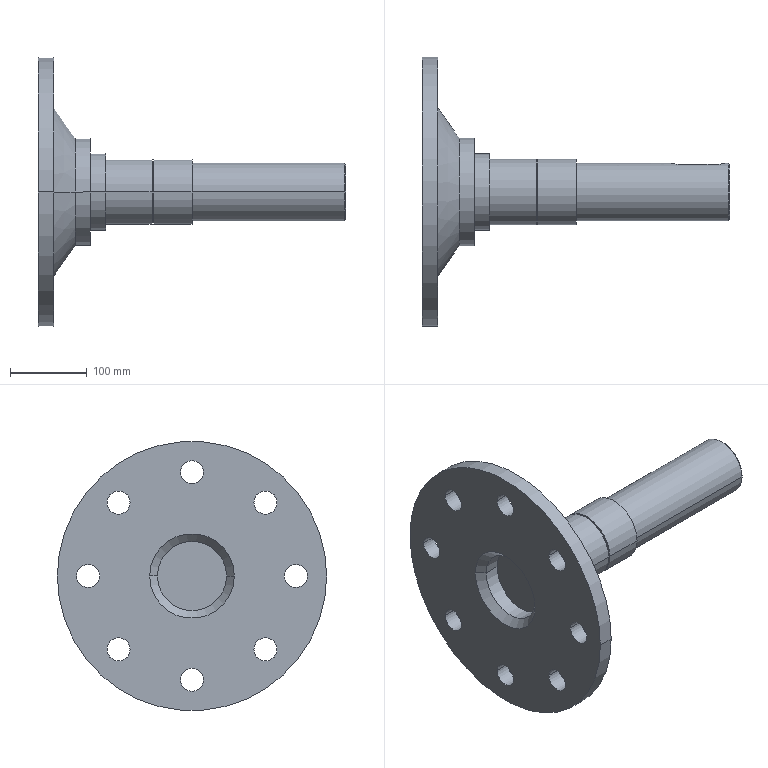Part | SolidWorks | features ICE 3, Chamfer 2, Revolution 1 | 1 solid | 52 faces | box 400 x 350 x 350 mm | volume 4309933 mm3 | cylinder 34 | plane 12 | cone 6 | commonest cylinder face diameters 30 x16 85 x4 20 x2 75 x2 81 x2 90 x2